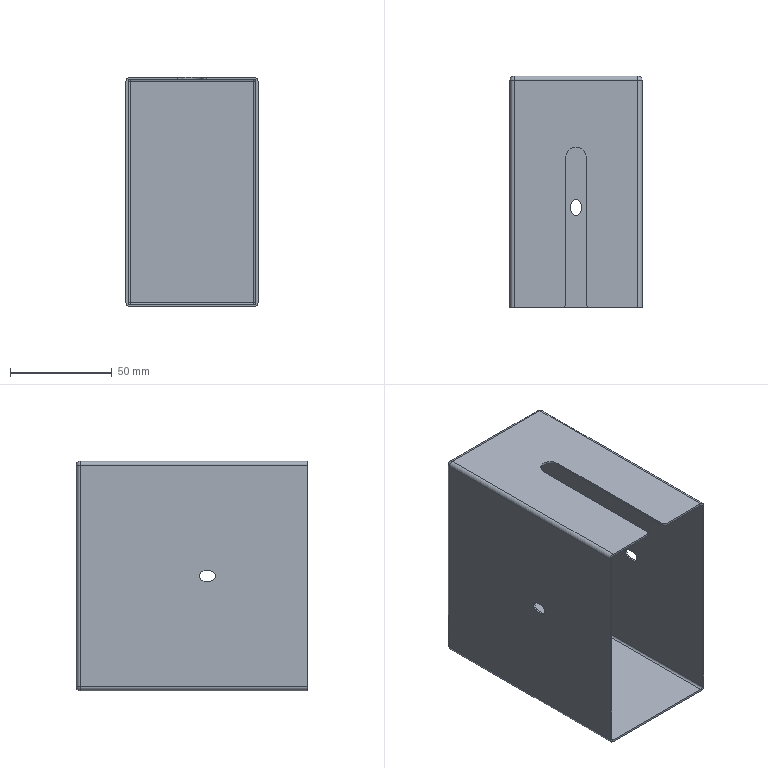Part | STEP file | ND25021-01-JDKM-01-BJ | 1 solid | 52 faces | box 65 x 114 x 113 mm | volume 45715 mm3 | cylinder 25 | plane 19 | sphere 8 | commonest cylinder face diameters 4 x10 2 x8 5 x6 10 x1